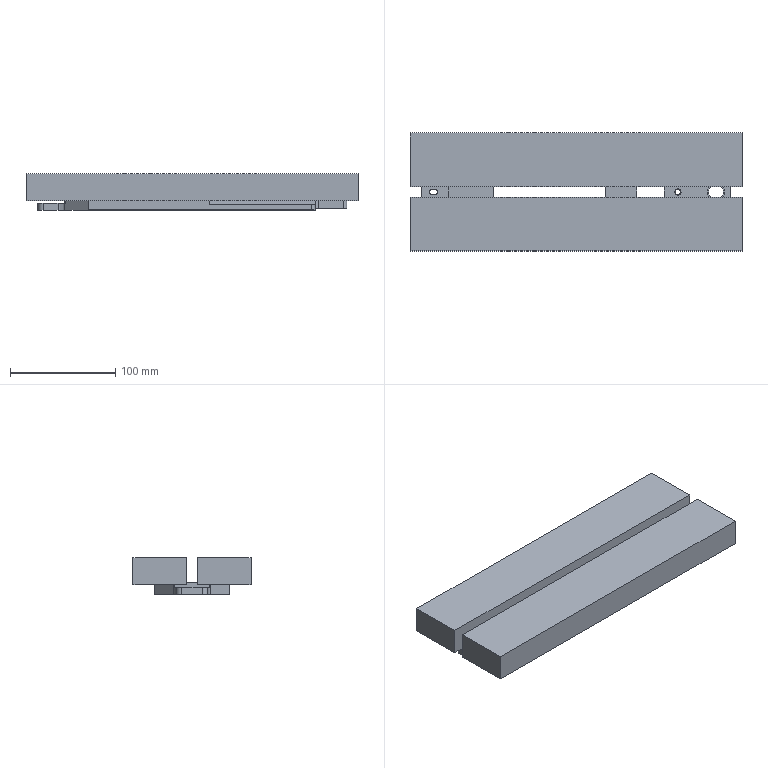NC program | NX | posted with a generic post | part box 315 x 112 x 34.85 mm
Lines 4523 to 5815 of 11462:
(PLANAR_MILL_7_COPY_1 , TOOL : D4精光)
N8984 T10 M6
N8986 G53
N8988 G17 G0 G90 X100.65 Y17.987 S4500 M3
N8990 G43 Z20. H10
N8992 Z0.3
N8994 G94 G1 Y18.214 Z0.284 F600.
N8996 X100.452 Y18.552 Z0.257
N8998 X100.114 Y18.75 Z0.229
N9000 X99.686 Z0.199
N9002 X99.349 Y18.552 Z0.172
N9004 X99.15 Y18.214 Z0.145
N9006 Y17.786 Z0.115
N9008 X99.349 Y17.448 Z0.087
N9010 X99.686 Y17.25 Z0.06
N9012 X100.114 Z0.03
N9014 X100.452 Y17.448 Z0.003
N9016 X100.65 Y17.786 Z-0.025
N9018 Y18.214 Z-0.055
N9020 X100.452 Y18.552 Z-0.082
N9022 X100.114 Y18.75 Z-0.109
N9024 X99.686 Z-0.139
N9026 X99.349 Y18.552 Z-0.167
N9028 X99.15 Y18.214 Z-0.194
N9030 Y17.786 Z-0.224
N9032 X99.349 Y17.448 Z-0.251
N9034 X99.686 Y17.25 Z-0.279
N9036 X100.114 Z-0.309
N9038 X100.452 Y17.448 Z-0.336
N9040 X100.65 Y17.786 Z-0.363
N9042 Y18.214 Z-0.393
N9044 X100.452 Y18.552 Z-0.421
N9046 X100.114 Y18.75 Z-0.448
N9048 X99.686 Z-0.478
N9050 X99.349 Y18.552 Z-0.506
N9052 X99.15 Y18.214 Z-0.533
N9054 Y17.786 Z-0.563
N9056 X99.349 Y17.448 Z-0.59
N9058 X99.686 Y17.25 Z-0.618
N9060 X100.114 Z-0.648
N9062 X100.452 Y17.448 Z-0.675
N9064 X100.65 Y17.786 Z-0.702
N9066 Y18.214 Z-0.732
N9068 X100.452 Y18.552 Z-0.76
N9070 X100.114 Y18.75 Z-0.787
N9072 X99.686 Z-0.817
N9074 X99.349 Y18.552 Z-0.844
N9076 X99.15 Y18.214 Z-0.872
N9078 Y17.786 Z-0.902
N9080 X99.349 Y17.448 Z-0.929
N9082 X99.686 Y17.25 Z-0.956
N9084 X100.114 Z-0.986
N9086 X100.452 Y17.448 Z-1.014
N9088 X100.65 Y17.786 Z-1.041
N9090 Y18.214 Z-1.071
N9092 X100.452 Y18.552 Z-1.098
N9094 X100.114 Y18.75 Z-1.126
N9096 X99.686 Z-1.156
N9098 X99.349 Y18.552 Z-1.183
N9100 X99.15 Y18.214 Z-1.21
N9102 Y17.786 Z-1.24
N9104 X99.349 Y17.448 Z-1.268
N9106 X99.686 Y17.25 Z-1.295
N9108 X100.114 Z-1.325
N9110 X100.452 Y17.448 Z-1.352
N9112 X100.65 Y17.786 Z-1.38
N9114 Y18.214 Z-1.41
N9116 X100.452 Y18.552 Z-1.437
N9118 X100.114 Y18.75 Z-1.465
N9120 X99.686 Z-1.494
N9122 X99.349 Y18.552 Z-1.522
N9124 X99.15 Y18.214 Z-1.549
N9126 Y17.786 Z-1.579
N9128 X99.349 Y17.448 Z-1.607
N9130 X99.686 Y17.25 Z-1.634
N9132 X100.114 Z-1.664
N9134 X100.452 Y17.448 Z-1.691
N9136 X100.65 Y17.786 Z-1.719
N9138 Y18.214 Z-1.749
N9140 X100.452 Y18.552 Z-1.776
N9142 X100.114 Y18.75 Z-1.803
N9144 X99.686 Z-1.833
N9146 X99.349 Y18.552 Z-1.861
N9148 X99.15 Y18.214 Z-1.888
N9150 Y17.786 Z-1.918
N9152 X99.349 Y17.448 Z-1.945
N9154 X99.686 Y17.25 Z-1.973
N9156 X100.114 Z-2.003
N9158 X100.452 Y17.448 Z-2.03
N9160 X100.65 Y17.786 Z-2.057
N9162 Y18.214 Z-2.087
N9164 X100.452 Y18.552 Z-2.115
N9166 X100.114 Y18.75 Z-2.142
N9168 X99.686 Z-2.172
N9170 X99.349 Y18.552 Z-2.199
N9172 X99.15 Y18.214 Z-2.227
N9174 Y17.786 Z-2.257
N9176 X99.349 Y17.448 Z-2.284
N9178 X99.686 Y17.25 Z-2.311
N9180 X100.114 Z-2.341
N9182 X100.452 Y17.448 Z-2.369
N9184 X100.65 Y17.786 Z-2.396
N9186 Y18.214 Z-2.426
N9188 X100.452 Y18.552 Z-2.453
N9190 X100.114 Y18.75 Z-2.481
N9192 X99.686 Z-2.511
N9194 X99.349 Y18.552 Z-2.538
N9196 X99.15 Y18.214 Z-2.566
N9198 Y17.786 Z-2.596
N9200 X99.349 Y17.448 Z-2.623
N9202 X99.686 Y17.25 Z-2.65
N9204 X100.114 Z-2.68
N9206 X100.452 Y17.448 Z-2.708
N9208 X100.65 Y17.786 Z-2.735
N9210 Y18.214 Z-2.765
N9212 X100.452 Y18.552 Z-2.792
N9214 X100.114 Y18.75 Z-2.82
N9216 X99.686 Z-2.85
N9218 X99.349 Y18.552 Z-2.877
N9220 X99.15 Y18.214 Z-2.904
N9222 Y17.786 Z-2.934
N9224 X99.349 Y17.448 Z-2.962
N9226 X99.686 Y17.25 Z-2.989
N9228 X100.114 Z-3.019
N9230 X100.452 Y17.448 Z-3.046
N9232 X100.65 Y17.786 Z-3.074
N9234 Y18.214 Z-3.104
N9236 X100.452 Y18.552 Z-3.131
N9238 X100.114 Y18.75 Z-3.158
N9240 X99.686 Z-3.188
N9242 X99.349 Y18.552 Z-3.216
N9244 X99.15 Y18.214 Z-3.243
N9246 Y17.786 Z-3.273
N9248 X99.349 Y17.448 Z-3.3
N9250 X99.686 Y17.25 Z-3.328
N9252 X100.114 Z-3.358
N9254 X100.452 Y17.448 Z-3.385
N9256 X100.65 Y17.786 Z-3.412
N9258 Y18.214 Z-3.442
N9260 X100.452 Y18.552 Z-3.47
N9262 X100.114 Y18.75 Z-3.497
N9264 X99.686 Z-3.527
N9266 X99.349 Y18.552 Z-3.555
N9268 X99.15 Y18.214 Z-3.582
N9270 Y17.786 Z-3.612
N9272 X99.349 Y17.448 Z-3.639
N9274 X99.686 Y17.25 Z-3.667
N9276 X100.114 Z-3.697
N9278 X100.452 Y17.448 Z-3.724
N9280 X100.65 Y17.786 Z-3.751
N9282 Y18.214 Z-3.781
N9284 X100.452 Y18.552 Z-3.809
N9286 X100.114 Y18.75 Z-3.836
N9288 X99.686 Z-3.866
N9290 X99.349 Y18.552 Z-3.893
N9292 X99.15 Y18.214 Z-3.921
N9294 Y17.786 Z-3.951
N9296 X99.349 Y17.448 Z-3.978
N9298 X99.686 Y17.25 Z-4.005
N9300 X100.114 Z-4.035
N9302 X100.452 Y17.448 Z-4.063
N9304 X100.65 Y17.786 Z-4.09
N9306 Y18.214 Z-4.12
N9308 X100.452 Y18.552 Z-4.147
N9310 X100.114 Y18.75 Z-4.175
N9312 X99.686 Z-4.205
N9314 X99.349 Y18.552 Z-4.232
N9316 X99.15 Y18.214 Z-4.259
N9318 Y17.786 Z-4.289
N9320 X99.349 Y17.448 Z-4.317
N9322 X99.686 Y17.25 Z-4.344
N9324 X100.114 Z-4.374
N9326 X100.452 Y17.448 Z-4.401
N9328 X100.65 Y17.786 Z-4.429
N9330 Y18.214 Z-4.459
N9332 X100.452 Y18.552 Z-4.486
N9334 X100.114 Y18.75 Z-4.514
N9336 X99.686 Z-4.543
N9338 X99.349 Y18.552 Z-4.571
N9340 X99.15 Y18.214 Z-4.598
N9342 Y17.786 Z-4.628
N9344 X99.349 Y17.448 Z-4.656
N9346 X99.686 Y17.25 Z-4.683
N9348 X100.114 Z-4.713
N9350 X100.452 Y17.448 Z-4.74
N9352 X100.65 Y17.786 Z-4.768
N9354 Y18.214 Z-4.798
N9356 X100.452 Y18.552 Z-4.825
N9358 X100.114 Y18.75 Z-4.852
N9360 X99.686 Z-4.882
N9362 X99.349 Y18.552 Z-4.91
N9364 X99.15 Y18.214 Z-4.937
N9366 Y17.786 Z-4.967
N9368 X99.349 Y17.448 Z-4.994
N9370 X99.686 Y17.25 Z-5.022
N9372 X100.114 Z-5.052
N9374 X100.452 Y17.448 Z-5.079
N9376 X100.65 Y17.786 Z-5.106
N9378 Y18.214 Z-5.136
N9380 X100.452 Y18.552 Z-5.164
N9382 X100.114 Y18.75 Z-5.191
N9384 X99.686 Z-5.221
N9386 X99.349 Y18.552 Z-5.248
N9388 X99.15 Y18.214 Z-5.276
N9390 Y17.786 Z-5.306
N9392 X99.349 Y17.448 Z-5.333
N9394 X99.686 Y17.25 Z-5.36
N9396 X100.114 Z-5.39
N9398 X100.452 Y17.448 Z-5.418
N9400 X100.65 Y17.786 Z-5.445
N9402 Y18.214 Z-5.475
N9404 X100.452 Y18.552 Z-5.502
N9406 X100.114 Y18.75 Z-5.53
N9408 X99.686 Z-5.56
N9410 X99.349 Y18.552 Z-5.587
N9412 X99.15 Y18.214 Z-5.615
N9414 Y17.786 Z-5.645
N9416 X99.349 Y17.448 Z-5.672
N9418 X99.686 Y17.25 Z-5.699
N9420 X100.114 Z-5.729
N9422 X100.452 Y17.448 Z-5.757
N9424 X100.65 Y17.786 Z-5.784
N9426 Y18.214 Z-5.814
N9428 X100.452 Y18.552 Z-5.841
N9430 X100.114 Y18.75 Z-5.869
N9432 X99.686 Z-5.899
N9434 X99.349 Y18.552 Z-5.926
N9436 X99.15 Y18.214 Z-5.953
N9438 Y17.786 Z-5.983
N9440 X99.349 Y17.448 Z-6.011
N9442 X99.686 Y17.25 Z-6.038
N9444 X100.114 Z-6.068
N9446 X100.452 Y17.448 Z-6.095
N9448 X100.65 Y17.786 Z-6.123
N9450 Y18.214 Z-6.153
N9452 X100.452 Y18.552 Z-6.18
N9454 X100.114 Y18.75 Z-6.207
N9456 X99.686 Z-6.237
N9458 X99.349 Y18.552 Z-6.265
N9460 X99.15 Y18.214 Z-6.292
N9462 Y17.786 Z-6.322
N9464 X99.349 Y17.448 Z-6.349
N9466 X99.686 Y17.25 Z-6.377
N9468 X100.114 Z-6.407
N9470 X100.452 Y17.448 Z-6.434
N9472 X100.65 Y17.786 Z-6.462
N9474 Y18.214 Z-6.491
N9476 X100.452 Y18.552 Z-6.519
N9478 X100.114 Y18.75 Z-6.546
N9480 X99.686 Z-6.576
N9482 X99.349 Y18.552 Z-6.604
N9484 X99.15 Y18.214 Z-6.631
N9486 Y17.786 Z-6.661
N9488 X99.349 Y17.448 Z-6.688
N9490 X99.686 Y17.25 Z-6.716
N9492 X100.114 Z-6.746
N9494 X100.452 Y17.448 Z-6.773
N9496 X100.65 Y17.786 Z-6.8
N9498 Y18.214 Z-6.83
N9500 X100.452 Y18.552 Z-6.858
N9502 X100.114 Y18.75 Z-6.885
N9504 X99.686 Z-6.915
N9506 X99.349 Y18.552 Z-6.942
N9508 X99.15 Y18.214 Z-6.97
N9510 Y17.786 Z-7.
N9512 X99.349 Y17.448 Z-7.027
N9514 X99.686 Y17.25 Z-7.054
N9516 X100.114 Z-7.084
N9518 X100.452 Y17.448 Z-7.112
N9520 X100.65 Y17.786 Z-7.139
N9522 Y18.214 Z-7.169
N9524 X100.452 Y18.552 Z-7.196
N9526 X100.114 Y18.75 Z-7.224
N9528 X99.686 Z-7.254
N9530 X99.349 Y18.552 Z-7.281
N9532 X99.15 Y18.214 Z-7.308
N9534 Y17.786 Z-7.338
N9536 X99.349 Y17.448 Z-7.366
N9538 X99.686 Y17.25 Z-7.393
N9540 X100.114 Z-7.423
N9542 X100.452 Y17.448 Z-7.45
N9544 X100.65 Y17.786 Z-7.478
N9546 Y18.214 Z-7.508
N9548 X100.452 Y18.552 Z-7.535
N9550 X100.114 Y18.75 Z-7.563
N9552 X99.686 Z-7.593
N9554 X99.349 Y18.552 Z-7.62
N9556 X99.15 Y18.214 Z-7.647
N9558 Y17.786 Z-7.677
N9560 X99.349 Y17.448 Z-7.705
N9562 X99.686 Y17.25 Z-7.732
N9564 X100.114 Z-7.762
N9566 X100.452 Y17.448 Z-7.789
N9568 X100.65 Y17.786 Z-7.817
N9570 Y18.214 Z-7.847
N9572 X100.452 Y18.552 Z-7.874
N9574 X100.114 Y18.75 Z-7.901
N9576 X99.686 Z-7.931
N9578 X99.349 Y18.552 Z-7.959
N9580 X99.15 Y18.214 Z-7.986
N9582 Y17.786 Z-8.016
N9584 X99.349 Y17.448 Z-8.043
N9586 X99.686 Y17.25 Z-8.071
N9588 X100.114 Z-8.101
N9590 X100.452 Y17.448 Z-8.128
N9592 X100.65 Y17.786 Z-8.155
N9594 Y18.214 Z-8.185
N9596 X100.452 Y18.552 Z-8.213
N9598 X100.114 Y18.75 Z-8.24
N9600 X99.686 Z-8.27
N9602 X99.349 Y18.552 Z-8.297
N9604 X99.15 Y18.214 Z-8.325
N9606 Y17.786 Z-8.355
N9608 X99.349 Y17.448 Z-8.382
N9610 X99.686 Y17.25 Z-8.409
N9612 X100.114 Z-8.439
N9614 X100.452 Y17.448 Z-8.467
N9616 X100.65 Y17.786 Z-8.494
N9618 Y18.214 Z-8.524
N9620 X100.452 Y18.552 Z-8.552
N9622 X100.114 Y18.75 Z-8.579
N9624 X99.686 Z-8.609
N9626 X99.349 Y18.552 Z-8.636
N9628 X99.15 Y18.214 Z-8.664
N9630 Y17.786 Z-8.694
N9632 X99.349 Y17.448 Z-8.721
N9634 X99.686 Y17.25 Z-8.748
N9636 X100.114 Z-8.778
N9638 X100.452 Y17.448 Z-8.806
N9640 X100.65 Y17.786 Z-8.833
N9642 Y18.214 Z-8.863
N9644 X100.452 Y18.552 Z-8.89
N9646 X100.114 Y18.75 Z-8.918
N9648 X99.686 Z-8.948
N9650 X99.349 Y18.552 Z-8.975
N9652 X99.15 Y18.214 Z-9.002
N9654 Y17.786 Z-9.032
N9656 X99.349 Y17.448 Z-9.06
N9658 X99.686 Y17.25 Z-9.087
N9660 X100.114 Z-9.117
N9662 X100.452 Y17.448 Z-9.144
N9664 X100.65 Y17.786 Z-9.172
N9666 Y18.214 Z-9.202
N9668 X100.452 Y18.552 Z-9.229
N9670 X100.114 Y18.75 Z-9.256
N9672 X99.686 Z-9.286
N9674 X99.349 Y18.552 Z-9.314
N9676 X99.15 Y18.214 Z-9.341
N9678 Y17.786 Z-9.371
N9680 X99.349 Y17.448 Z-9.398
N9682 X99.686 Y17.25 Z-9.426
N9684 X100.114 Z-9.456
N9686 X100.452 Y17.448 Z-9.483
N9688 X100.65 Y17.786 Z-9.511
N9690 Y18.214 Z-9.54
N9692 X100.452 Y18.552 Z-9.568
N9694 X100.114 Y18.75 Z-9.595
N9696 X99.686 Z-9.625
N9698 X99.349 Y18.552 Z-9.653
N9700 X99.15 Y18.214 Z-9.68
N9702 Y17.786 Z-9.71
N9704 X99.349 Y17.448 Z-9.737
N9706 X99.686 Y17.25 Z-9.765
N9708 X100.114 Z-9.795
N9710 X100.452 Y17.448 Z-9.822
N9712 X100.65 Y17.786 Z-9.849
N9714 Y18.214 Z-9.879
N9716 X100.452 Y18.552 Z-9.907
N9718 X100.114 Y18.75 Z-9.934
N9720 X99.686 Z-9.964
N9722 X99.349 Y18.552 Z-9.991
N9724 X99.15 Y18.214 Z-10.019
N9726 Y17.786 Z-10.049
N9728 X99.349 Y17.448 Z-10.076
N9730 X99.686 Y17.25 Z-10.103
N9732 X100.114 Z-10.133
N9734 X100.452 Y17.448 Z-10.161
N9736 X100.65 Y17.786 Z-10.188
N9738 Y18.214 Z-10.218
N9740 X100.452 Y18.552 Z-10.245
N9742 X100.114 Y18.75 Z-10.273
N9744 X99.686 Z-10.303
N9746 X99.349 Y18.552 Z-10.33
N9748 X99.15 Y18.214 Z-10.357
N9750 Y17.786 Z-10.387
N9752 X99.349 Y17.448 Z-10.415
N9754 X99.686 Y17.25 Z-10.442
N9756 X100.114 Z-10.472
N9758 X100.452 Y17.448 Z-10.499
N9760 X100.65 Y17.786 Z-10.527
N9762 Y18.214 Z-10.557
N9764 X100.452 Y18.552 Z-10.584
N9766 X100.114 Y18.75 Z-10.612
N9768 X99.686 Z-10.642
N9770 X99.349 Y18.552 Z-10.669
N9772 X99.15 Y18.214 Z-10.696
N9774 Y17.786 Z-10.726
N9776 X99.349 Y17.448 Z-10.754
N9778 X99.686 Y17.25 Z-10.781
N9780 X100.114 Z-10.811
N9782 X100.452 Y17.448 Z-10.838
N9784 X100.65 Y17.786 Z-10.866
N9786 Y18.214 Z-10.896
N9788 X100.452 Y18.552 Z-10.923
N9790 X100.114 Y18.75 Z-10.95
N9792 X99.686 Z-10.98
N9794 X99.349 Y18.552 Z-11.008
N9796 X99.15 Y18.214 Z-11.035
N9798 Y18. Z-11.05
N9800 G3 X99.9 Y17.25 R0.75
N9802 X99.15 Y18. R-0.75
N9804 G1 Z-10.75
N9806 G0 Z20.
N9808 M5
(PLANAR_MILL_1 , TOOL : D6精光)
N9810 T09 M6
N9812 G53
N9814 G17 G0 G90 X115.623 Y-41.542 S5500 M3
N9816 G43 Z20. H9
N9818 Z-8.85
N9820 G94 G1 Z-11.85 F1000.
N9822 G41 X115.71 Y-41.05 D9
N9824 G3 X113.71 Y-39.05 R2.
N9826 G1 X-98.29
N9828 G2 X-100.252 Y-38.335 R3.05
N9830 G1 X-122.641 Y-19.528
N9832 G3 X-127.111 Y-17.9 R6.95
N9834 G1 X-141.29
N9836 G2 X-149.34 Y-9.85 R8.05
N9838 G1 Y9.85
N9840 G2 X-141.29 Y17.9 R8.05
N9842 G1 X-127.111
N9844 G3 X-122.641 Y19.528 R6.95
N9846 G1 X-100.252 Y38.335
N9848 G2 X-98.29 Y39.05 R3.05
N9850 G1 X113.71
N9852 G2 X119.76 Y33. R6.05
N9854 G1 Y15.55
N9856 X143.71
N9858 G2 X149.76 Y9.5 R6.05
N9860 G1 Y-9.5
N9862 G2 X143.71 Y-15.55 R6.05
N9864 G1 X119.76
N9866 Y-33.
N9868 G2 X113.71 Y-39.05 R6.05
N9870 G3 X111.71 Y-41.05 R2.
N9872 G40
N9874 G1 X111.797 Y-41.542
N9876 X115.623 Y-41.492
N9878 G41 X115.71 Y-41.
N9880 G3 X113.71 Y-39. R2.
N9882 G1 X-98.29
N9884 G2 X-100.22 Y-38.297 R3.
N9886 G1 X-122.609 Y-19.49
N9888 G3 X-127.111 Y-17.85 R7.
N9890 G1 X-141.29
N9892 G2 X-149.29 Y-9.85 R8.
N9894 G1 Y9.85
N9896 G2 X-141.29 Y17.85 R8.
N9898 G1 X-127.111
N9900 G3 X-122.609 Y19.49 R7.
N9902 G1 X-100.22 Y38.297
N9904 G2 X-98.29 Y39. R3.
N9906 G1 X113.71
N9908 G2 X119.71 Y33. R6.
N9910 G1 Y15.5
N9912 X143.71
N9914 G2 X149.71 Y9.5 R6.
N9916 G1 Y-9.5
N9918 G2 X143.71 Y-15.5 R6.
N9920 G1 X119.71
N9922 Y-33.
N9924 G2 X113.71 Y-39. R6.
N9926 G3 X111.71 Y-41. R2.
N9928 G1 Y-41.05
N9930 G40
N9932 X111.797 Y-41.542
N9934 Z-8.85
N9936 G0 Z20.
(PLANAR_MILL_1_COPY , TOOL : D6精光)
N9938 X130.374 Y0.913 H29
N9940 Z-8.85
N9942 G1 Z-11.85 F100.
N9944 G41 X129.882 Y1. D29
N9946 X129.71
N9948 G3 X128.71 Y0. R1.
N9950 X132.71 Y-4. R4.
N9952 X128.71 Y0. R-4.
N9954 X129.71 Y-1. R1.
N9956 G40
N9958 G1 X130.202 Y-0.913
N9960 Y0.913
N9962 G41 X129.71 Y1.
N9964 G3 X128.71 Y0. R1.
N9966 X132.71 Y-4. R4.
N9968 X128.71 Y0. R-4.
N9970 X129.71 Y-1. R1.
N9972 G1 X129.882
N9974 G40
N9976 X130.374 Y-0.913
N9978 Z-8.85
N9980 G0 Z20.
(PLANAR_MILL_1_COPY_COPY_1 , TOOL : D6精光)
N9982 X18.643 Y20.424 H9
N9984 Z-8.85
N9986 G1 Z-11.85 F600.
N9988 G41 X18.73 Y20.916 D9
N9990 Y21.
N9992 G3 X17.73 Y22. R1.
N9994 G1 X-68.31
N9996 G3 X-75.31 Y15. R7.
N9998 G1 Y-15.
N10000 G3 X-68.31 Y-22. R7.
N10002 G1 X17.73
N10004 G3 X24.73 Y-15. R7.
N10006 G1 Y15.
N10008 G3 X17.73 Y22. R7.
N10010 X16.73 Y21. R1.
N10012 G40
N10014 G1 X16.817 Y20.508
N10016 Z-8.85
N10018 G0 Z20.
(PLANAR_MILL_1_COPY_COPY , TOOL : D6精光)
N10020 X129.092 Y0.913
N10022 Z-1.
N10024 G1 Z-4. F100.
N10026 G41 X128.6 Y1.
N10028 X128.48
N10030 G3 X127.48 Y0. R1.
N10032 X132.71 Y-5.23 R5.23
N10034 X127.48 Y0. R-5.23
N10036 X128.48 Y-1. R1.
N10038 G40
N10040 G1 X128.972 Y-0.913
N10042 X128.952 Y0.913
N10044 G41 X128.46 Y1.
N10046 G3 X127.46 Y0. R1.
N10048 X132.71 Y-5.25 R5.25
N10050 X127.46 Y0. R-5.25
N10052 X128.46 Y-1. R1.
N10054 G1 X128.579
N10056 G40
N10058 X129.072 Y-0.913
N10060 Z-1.
N10062 G0 Z20.
(FLOOR_WALL , TOOL : D6精光)
N10064 X101.257 Y41.
N10066 Z-2.
N10068 G1 Z-5. F600.
N10070 Y34.5
N10072 X113.71
N10074 G2 X115.21 Y33. R1.5
N10076 G1 Y21.171
N10078 X41.898 Y34.5
N10080 X101.257
N10082 Y30.
N10084 X110.71
N10086 Y26.563
N10088 X91.804 Y30.
N10090 X89.206 Y31.5
N10092 X75.169
N10094 X88.979 Y28.989
N10096 G2 X89.206 Y31.5 R3.
N10098 G1 X91.804 Y30.
N10100 X101.257
N10102 X102.257
N10104 Y41.
N10106 Z-2.
N10108 G0 Z20.
N10110 X101.257 Y-41.
N10112 Z-2.
N10114 G1 Z-5.
N10116 Y-34.5
N10118 X41.898
N10120 X115.21 Y-21.171
N10122 Y-33.
N10124 G2 X113.71 Y-34.5 R1.5
N10126 G1 X101.257
N10128 Y-30.
N10130 X91.804
N10132 X88.979 Y-28.989
N10134 X75.169 Y-31.5
N10136 X89.206
N10138 G2 X88.979 Y-28.989 R3.
N10140 G1 X91.804 Y-30.
N10142 X110.71 Y-26.563
N10144 Y-30.
N10146 X101.257
N10148 X100.257
N10150 Y-41.
N10152 Z-2.
N10154 G0 Z20.
(PLANAR_MILL_6 , TOOL : D6精光)
N10156 X12.842 Y39.841
N10158 Z-1.995
N10160 G1 Z-4.995 F800.
N10162 G41 X13.311 Y39.667
N10164 X17.247 Y38.952
N10166 X117.247 Y20.77
N10168 X121.182 Y20.054
N10170 G40
N10172 X121.682 Y20.052
N10174 Z-1.995
N10176 G0 Z20.
N10178 Y-20.052
N10180 Z-1.995
N10182 G1 Z-4.995
N10184 G41 X121.182 Y-20.054
N10186 X117.247 Y-20.77
N10188 X17.247 Y-38.952
N10190 X13.311 Y-39.667
N10192 G40
N10194 X12.842 Y-39.841
N10196 Z-1.995
N10198 G0 Z20.
(FLOOR_WALL_1 , TOOL : D6精光)
N10200 X-151.29 Y0.
N10202 Z-1.
N10204 G1 Z-4. F600.
N10206 X-144.79
N10208 Y9.85
N10210 G2 X-141.29 Y13.35 R3.5
N10212 G1 X-127.111
N10214 G3 X-123.5 Y13.932 R11.5
N10216 G1 Y-13.932
N10218 G3 X-127.111 Y-13.35 R11.5
N10220 G1 X-141.29
N10222 G2 X-144.79 Y-9.85 R3.5
N10224 G1 Y0.
N10226 X-140.29
N10228 Y8.85
N10230 X-128.
N10232 Y-8.85
N10234 X-140.29
N10236 Y0.
N10238 X-135.79
N10240 Y4.35
N10242 X-132.5
N10244 Y-4.35
N10246 X-135.79
N10248 Y0.
N10250 Y1.
N10252 X-137.79
N10254 Z-1.
N10256 G0 Z20.
(PLANAR_MILL_6_COPY , TOOL : D6精光)
N10258 X-121.854 Y-23.379
N10260 Z-0.995
N10262 G1 Z-3.995 F800.
N10264 G41 X-121.471 Y-23.058
N10266 G3 X-121.716 Y-20.24 R2.
N10268 G2 X-123.5 Y-16.412 R5.
N10270 G1 Y16.412
N10272 G2 X-121.716 Y20.24 R5.
N10274 G3 X-121.471 Y23.058 R2.
N10276 G40
N10278 G1 X-121.854 Y23.379
N10280 Z-0.995
N10282 G0 Z20.
(PLANAR_MILL_1_COPY_1 , TOOL : D6精光)
N10284 X-139.377 Y-20.392
N10286 Z-8.85
N10288 G1 Z-11.85 F1000.
N10290 G41 X-139.29 Y-19.9
N10292 G3 X-141.29 Y-17.9 R2.
N10294 G2 X-149.34 Y-9.85 R8.05
N10296 G1 Y9.85
N10298 G2 X-141.29 Y17.9 R8.05
N10300 G3 X-139.29 Y19.9 R2.
N10302 G40
N10304 G1 X-139.377 Y20.392
N10306 Z-8.85
N10308 G0 Z20.
N10310 Y-20.392
N10312 Z-8.85
N10314 G1 Z-11.85
N10316 G41 X-139.29 Y-19.9
N10318 Y-19.85
N10320 G3 X-141.29 Y-17.85 R2.
N10322 G2 X-149.29 Y-9.85 R8.
N10324 G1 Y9.85
N10326 G2 X-141.29 Y17.85 R8.
N10328 G3 X-139.29 Y19.85 R2.
N10330 G1 Y19.9
N10332 G40
N10334 X-139.377 Y20.392
N10336 Z-8.85
N10338 G0 Z20.
N10340 M5
(PLANAR_MILL_7 , TOOL : D4精光)
N10342 T10 M6
N10344 G53
N10346 G17 G0 G90 X96.27 Y-0.151 S4500 M3
N10348 G43 Z20. H10
N10350 Z-0.2
N10352 G94 G1 Y-0.165 Z-0.201 F600.
N10354 X96.545 Y-0.44 Z-0.228
N10356 X96.875 Z-0.251
N10358 X97.15 Y-0.165 Z-0.278
N10360 Y0.165 Z-0.302
N10362 X96.875 Y0.44 Z-0.329
N10364 X96.545 Z-0.352
N10366 X96.27 Y0.165 Z-0.379
N10368 Y-0.165 Z-0.402
N10370 X96.545 Y-0.44 Z-0.429
N10372 X96.875 Z-0.452
N10374 X97.15 Y-0.165 Z-0.48
N10376 Y0.165 Z-0.503
N10378 X96.875 Y0.44 Z-0.53
N10380 X96.545 Z-0.553
N10382 X96.27 Y0.165 Z-0.58
N10384 Y-0.165 Z-0.603
N10386 X96.545 Y-0.44 Z-0.63
N10388 X96.875 Z-0.654
N10390 X97.15 Y-0.165 Z-0.681
N10392 Y0.165 Z-0.704
N10394 X96.875 Y0.44 Z-0.731
N10396 X96.545 Z-0.754
N10398 X96.27 Y0.165 Z-0.781
N10400 Y-0.165 Z-0.804
N10402 X96.545 Y-0.44 Z-0.832
N10404 X96.875 Z-0.855
N10406 X97.15 Y-0.165 Z-0.882
N10408 Y0.165 Z-0.905
N10410 X96.875 Y0.44 Z-0.932
N10412 X96.545 Z-0.955
N10414 X96.27 Y0.165 Z-0.982
N10416 Y-0.165 Z-1.005
N10418 X96.545 Y-0.44 Z-1.033
N10420 X96.875 Z-1.056
N10422 X97.15 Y-0.165 Z-1.083
N10424 Y0.165 Z-1.106
N10426 X96.875 Y0.44 Z-1.133
N10428 X96.545 Z-1.156
N10430 X96.27 Y0.165 Z-1.184
N10432 Y-0.165 Z-1.207
N10434 X96.545 Y-0.44 Z-1.234
N10436 X96.875 Z-1.257
N10438 X97.15 Y-0.165 Z-1.284
N10440 Y0.165 Z-1.307
N10442 X96.875 Y0.44 Z-1.334
N10444 X96.545 Z-1.357
N10446 X96.27 Y0.165 Z-1.385
N10448 Y-0.165 Z-1.408
N10450 X96.545 Y-0.44 Z-1.435
N10452 X96.875 Z-1.458
N10454 X97.15 Y-0.165 Z-1.485
N10456 Y0.165 Z-1.508
N10458 X96.875 Y0.44 Z-1.535
N10460 X96.545 Z-1.559
N10462 X96.27 Y0.165 Z-1.586
N10464 Y-0.165 Z-1.609
N10466 X96.545 Y-0.44 Z-1.636
N10468 X96.875 Z-1.659
N10470 X97.15 Y-0.165 Z-1.686
N10472 Y0.165 Z-1.709
N10474 X96.875 Y0.44 Z-1.737
N10476 X96.545 Z-1.76
N10478 X96.27 Y0.165 Z-1.787
N10480 Y-0.165 Z-1.81
N10482 X96.545 Y-0.44 Z-1.837
N10484 X96.875 Z-1.86
N10486 X97.15 Y-0.165 Z-1.887
N10488 Y0.165 Z-1.911
N10490 X96.875 Y0.44 Z-1.938
N10492 X96.545 Z-1.961
N10494 X96.27 Y0.165 Z-1.988
N10496 Y-0.165 Z-2.011
N10498 X96.545 Y-0.44 Z-2.038
N10500 X96.875 Z-2.061
N10502 X97.15 Y-0.165 Z-2.089
N10504 Y0.165 Z-2.112
N10506 X96.875 Y0.44 Z-2.139
N10508 X96.545 Z-2.162
N10510 X96.27 Y0.165 Z-2.189
N10512 Y-0.165 Z-2.212
N10514 X96.545 Y-0.44 Z-2.239
N10516 X96.875 Z-2.263
N10518 X97.15 Y-0.165 Z-2.29
N10520 Y0.165 Z-2.313
N10522 X96.875 Y0.44 Z-2.34
N10524 X96.545 Z-2.363
N10526 X96.27 Y0.165 Z-2.39
N10528 Y-0.165 Z-2.413
N10530 X96.545 Y-0.44 Z-2.441
N10532 X96.875 Z-2.464
N10534 X97.15 Y-0.165 Z-2.491
N10536 Y0.165 Z-2.514
N10538 X96.875 Y0.44 Z-2.541
N10540 X96.545 Z-2.564
N10542 X96.27 Y0.165 Z-2.591
N10544 Y-0.165 Z-2.614
N10546 X96.545 Y-0.44 Z-2.642
N10548 X96.875 Z-2.665
N10550 X97.15 Y-0.165 Z-2.692
N10552 Y0.165 Z-2.715
N10554 X96.875 Y0.44 Z-2.742
N10556 X96.545 Z-2.765
N10558 X96.27 Y0.165 Z-2.792
N10560 Y-0.165 Z-2.816
N10562 X96.545 Y-0.44 Z-2.843
N10564 X96.875 Z-2.866
N10566 X97.15 Y-0.165 Z-2.893
N10568 Y0.165 Z-2.916
N10570 X96.875 Y0.44 Z-2.943
N10572 X96.545 Z-2.966
N10574 X96.27 Y0.165 Z-2.994
N10576 Y-0.165 Z-3.017
N10578 X96.545 Y-0.44 Z-3.044
N10580 X96.875 Z-3.067
N10582 X97.15 Y-0.165 Z-3.094
N10584 Y0.165 Z-3.117
N10586 X96.875 Y0.44 Z-3.144
N10588 X96.545 Z-3.168
N10590 X96.27 Y0.165 Z-3.195
N10592 Y-0.165 Z-3.218
N10594 X96.545 Y-0.44 Z-3.245
N10596 X96.875 Z-3.268
N10598 X97.15 Y-0.165 Z-3.295
N10600 Y0.165 Z-3.318
N10602 X96.875 Y0.44 Z-3.346
N10604 X96.545 Z-3.369
N10606 X96.27 Y0.165 Z-3.396
N10608 Y-0.165 Z-3.419
N10610 X96.545 Y-0.44 Z-3.446
N10612 X96.875 Z-3.469
N10614 X97.15 Y-0.165 Z-3.496
N10616 Y0.165 Z-3.52
N10618 X96.875 Y0.44 Z-3.547
N10620 X96.545 Z-3.57
N10622 X96.27 Y0.165 Z-3.597
N10624 Y-0.165 Z-3.62
N10626 X96.545 Y-0.44 Z-3.647
N10628 X96.875 Z-3.67
N10630 X97.15 Y-0.165 Z-3.698
N10632 Y0.165 Z-3.721
N10634 X96.875 Y0.44 Z-3.748
N10636 X96.545 Z-3.771
N10638 X96.27 Y0.165 Z-3.798
N10640 Y-0.165 Z-3.821
N10642 X96.545 Y-0.44 Z-3.848
N10644 X96.875 Z-3.871
N10646 X97.15 Y-0.165 Z-3.899
N10648 Y0.165 Z-3.922
N10650 X96.875 Y0.44 Z-3.949
N10652 X96.545 Z-3.972
N10654 X96.27 Y0.165 Z-3.999
N10656 Y-0.165 Z-4.022
N10658 X96.545 Y-0.44 Z-4.049
N10660 X96.875 Z-4.073
N10662 X97.15 Y-0.165 Z-4.1
N10664 Y0.165 Z-4.123
N10666 X96.875 Y0.44 Z-4.15
N10668 X96.545 Z-4.173
N10670 X96.27 Y0.165 Z-4.2
N10672 Y-0.165 Z-4.223
N10674 X96.545 Y-0.44 Z-4.251
N10676 X96.875 Z-4.274
N10678 X97.15 Y-0.165 Z-4.301
N10680 Y0.165 Z-4.324
N10682 X96.875 Y0.44 Z-4.351
N10684 X96.545 Z-4.374
N10686 X96.27 Y0.165 Z-4.401
N10688 Y-0.165 Z-4.425
N10690 X96.545 Y-0.44 Z-4.452
N10692 X96.875 Z-4.475
N10694 X97.15 Y-0.165 Z-4.502
N10696 Y0.165 Z-4.525
N10698 X96.875 Y0.44 Z-4.552
N10700 X96.545 Z-4.575
N10702 X96.27 Y0.165 Z-4.603
N10704 Y-0.165 Z-4.626
N10706 X96.545 Y-0.44 Z-4.653
N10708 X96.875 Z-4.676
N10710 X97.15 Y-0.165 Z-4.703
N10712 Y0.165 Z-4.726
N10714 X96.875 Y0.44 Z-4.753
N10716 X96.545 Z-4.777
N10718 X96.27 Y0.165 Z-4.804
N10720 Y-0.165 Z-4.827
N10722 X96.545 Y-0.44 Z-4.854
N10724 X96.875 Z-4.877
N10726 X97.15 Y-0.165 Z-4.904
N10728 Y0.165 Z-4.927
N10730 X96.875 Y0.44 Z-4.955
N10732 X96.545 Z-4.978
N10734 X96.27 Y0.165 Z-5.005
N10736 Y-0.165 Z-5.028
N10738 X96.545 Y-0.44 Z-5.055
N10740 X96.875 Z-5.078
N10742 X97.15 Y-0.165 Z-5.105
N10744 Y0.165 Z-5.128
N10746 X96.875 Y0.44 Z-5.156
N10748 X96.545 Z-5.179
N10750 X96.27 Y0.165 Z-5.206
N10752 Y-0.165 Z-5.229
N10754 X96.545 Y-0.44 Z-5.256
N10756 X96.875 Z-5.279
N10758 X97.15 Y-0.165 Z-5.306
N10760 Y0.165 Z-5.33
N10762 X96.875 Y0.44 Z-5.357
N10764 X96.545 Z-5.38
N10766 X96.27 Y0.165 Z-5.407
N10768 Y-0.165 Z-5.43
N10770 X96.545 Y-0.44 Z-5.457
N10772 X96.875 Z-5.48
N10774 X97.15 Y-0.165 Z-5.508
N10776 Y0.165 Z-5.531
N10778 X96.875 Y0.44 Z-5.558
N10780 X96.545 Z-5.581
N10782 X96.27 Y0.165 Z-5.608
N10784 Y-0.165 Z-5.631
N10786 X96.545 Y-0.44 Z-5.658
N10788 X96.875 Z-5.682
N10790 X97.15 Y-0.165 Z-5.709
N10792 Y0.165 Z-5.732
N10794 X96.875 Y0.44 Z-5.759
N10796 X96.545 Z-5.782
N10798 X96.27 Y0.165 Z-5.809
N10800 Y-0.165 Z-5.832
N10802 X96.545 Y-0.44 Z-5.86
N10804 X96.875 Z-5.883
N10806 X97.15 Y-0.165 Z-5.91
N10808 Y0.165 Z-5.933
N10810 X96.875 Y0.44 Z-5.96
N10812 X96.545 Z-5.983
N10814 X96.27 Y0.165 Z-6.01
N10816 Y-0.165 Z-6.034
N10818 X96.545 Y-0.44 Z-6.061
N10820 X96.875 Z-6.084
N10822 X97.15 Y-0.165 Z-6.111
N10824 Y0.165 Z-6.134
N10826 X96.875 Y0.44 Z-6.161
N10828 X96.545 Z-6.184
N10830 X96.27 Y0.165 Z-6.212
N10832 Y-0.165 Z-6.235
N10834 X96.545 Y-0.44 Z-6.262
N10836 X96.875 Z-6.285
N10838 X97.15 Y-0.165 Z-6.312
N10840 Y0.165 Z-6.335
N10842 X96.875 Y0.44 Z-6.362
N10844 X96.545 Z-6.385
N10846 X96.27 Y0.165 Z-6.413
N10848 Y-0.165 Z-6.436
N10850 X96.545 Y-0.44 Z-6.463
N10852 X96.875 Z-6.486
N10854 X97.15 Y-0.165 Z-6.513
N10856 Y0.165 Z-6.536
N10858 X96.875 Y0.44 Z-6.564
N10860 X96.545 Z-6.587
N10862 X96.27 Y0.165 Z-6.614
N10864 Y-0.165 Z-6.637
N10866 X96.545 Y-0.44 Z-6.664
N10868 X96.875 Z-6.687
N10870 X97.15 Y-0.165 Z-6.714
N10872 Y0.165 Z-6.737
N10874 X96.875 Y0.44 Z-6.765
N10876 X96.545 Z-6.788
N10878 X96.27 Y0.165 Z-6.815
N10880 Y-0.165 Z-6.838
N10882 X96.545 Y-0.44 Z-6.865
N10884 X96.875 Z-6.888
N10886 X97.15 Y-0.165 Z-6.915
N10888 Y0.165 Z-6.939
N10890 X96.875 Y0.44 Z-6.966
N10892 X96.545 Z-6.989
N10894 X96.27 Y0.165 Z-7.016
N10896 Y-0.165 Z-7.039
N10898 X96.545 Y-0.44 Z-7.066
N10900 X96.875 Z-7.089
N10902 X97.15 Y-0.165 Z-7.117
N10904 Y0.165 Z-7.14
N10906 X96.875 Y0.44 Z-7.167
N10908 X96.545 Z-7.19
N10910 X96.27 Y0.165 Z-7.217
N10912 Y-0.165 Z-7.24
N10914 X96.545 Y-0.44 Z-7.267
N10916 X96.875 Z-7.291
N10918 X97.15 Y-0.165 Z-7.318
N10920 Y0.165 Z-7.341
N10922 X96.875 Y0.44 Z-7.368
N10924 X96.545 Z-7.391
N10926 X96.27 Y0.165 Z-7.418
N10928 Y-0.165 Z-7.441
N10930 X96.545 Y-0.44 Z-7.469
N10932 X96.875 Z-7.492
N10934 X97.15 Y-0.165 Z-7.519
N10936 Y0.165 Z-7.542
N10938 X96.875 Y0.44 Z-7.569
N10940 X96.545 Z-7.592
N10942 X96.27 Y0.165 Z-7.619
N10944 Y-0.165 Z-7.642
N10946 X96.545 Y-0.44 Z-7.67
N10948 X96.875 Z-7.693
N10950 X97.15 Y-0.165 Z-7.72
N10952 Y0.165 Z-7.743
N10954 X96.875 Y0.44 Z-7.77
N10956 X96.545 Z-7.793
N10958 X96.27 Y0.165 Z-7.821
N10960 Y-0.165 Z-7.844
N10962 X96.545 Y-0.44 Z-7.871
N10964 X96.875 Z-7.894
N10966 X97.15 Y-0.165 Z-7.921
N10968 Y0.165 Z-7.944
N10970 X96.875 Y0.44 Z-7.971
N10972 X96.545 Z-7.994
N10974 X96.27 Y0.165 Z-8.022
N10976 Y-0.165 Z-8.045
N10978 X96.545 Y-0.44 Z-8.072
N10980 X96.875 Z-8.095
N10982 X97.15 Y-0.165 Z-8.122
N10984 Y0.165 Z-8.145
N10986 X96.875 Y0.44 Z-8.172
N10988 X96.545 Z-8.196
N10990 X96.27 Y0.165 Z-8.223
N10992 Y-0.165 Z-8.246
N10994 X96.545 Y-0.44 Z-8.273
N10996 X96.875 Z-8.296
N10998 X97.15 Y-0.165 Z-8.323
N11000 Y0.165 Z-8.346
N11002 X96.875 Y0.44 Z-8.374
N11004 X96.545 Z-8.397
N11006 X96.27 Y0.165 Z-8.424
N11008 Y-0.165 Z-8.447
N11010 X96.545 Y-0.44 Z-8.474
N11012 X96.875 Z-8.497
N11014 X97.15 Y-0.165 Z-8.524
N11016 Y0.165 Z-8.548
N11018 X96.875 Y0.44 Z-8.575
N11020 X96.545 Z-8.598
N11022 X96.27 Y0.165 Z-8.625
N11024 Y-0.165 Z-8.648
N11026 X96.545 Y-0.44 Z-8.675
N11028 X96.875 Z-8.698
N11030 X97.15 Y-0.165 Z-8.726
N11032 Y0.165 Z-8.749
N11034 X96.875 Y0.44 Z-8.776
N11036 X96.545 Z-8.799
N11038 X96.27 Y0.165 Z-8.826
N11040 Y-0.165 Z-8.849
N11042 X96.545 Y-0.44 Z-8.876
N11044 X96.875 Z-8.9
N11046 X97.15 Y-0.165 Z-8.927
N11048 Y0.165 Z-8.95
N11050 X96.875 Y0.44 Z-8.977
N11052 X96.545 Z-9.
N11054 X96.27 Y0.165 Z-9.027
N11056 Y-0.165 Z-9.05
N11058 X96.545 Y-0.44 Z-9.078
N11060 X96.875 Z-9.101
N11062 X97.15 Y-0.165 Z-9.128
N11064 Y0.165 Z-9.151
N11066 X96.875 Y0.44 Z-9.178
N11068 X96.545 Z-9.201
N11070 X96.27 Y0.165 Z-9.228
N11072 Y-0.165 Z-9.251
N11074 X96.545 Y-0.44 Z-9.279
N11076 X96.875 Z-9.302
N11078 X97.15 Y-0.165 Z-9.329
N11080 Y0.165 Z-9.352
N11082 X96.875 Y0.44 Z-9.379
N11084 X96.545 Z-9.402
N11086 X96.27 Y0.165 Z-9.429
N11088 Y-0.165 Z-9.453
N11090 X96.545 Y-0.44 Z-9.48
N11092 X96.875 Z-9.503
N11094 X97.15 Y-0.165 Z-9.53
N11096 Y0.165 Z-9.553
N11098 X96.875 Y0.44 Z-9.58
N11100 X96.545 Z-9.603
N11102 X96.27 Y0.165 Z-9.631
N11104 Y-0.165 Z-9.654
N11106 X96.545 Y-0.44 Z-9.681
N11108 X96.875 Z-9.704
N11110 X97.15 Y-0.165 Z-9.731
N11112 Y0.165 Z-9.754
N11114 X96.875 Y0.44 Z-9.781
N11116 X96.545 Z-9.805
N11118 X96.27 Y0.165 Z-9.832
N11120 Y-0.165 Z-9.855
N11122 X96.545 Y-0.44 Z-9.882
N11124 X96.875 Z-9.905
N11126 X97.15 Y-0.165 Z-9.932
N11128 Y0.165 Z-9.955
N11130 X96.875 Y0.44 Z-9.983
N11132 X96.545 Z-10.006
N11134 X96.27 Y0.165 Z-10.033
N11136 Y-0.165 Z-10.056
N11138 X96.545 Y-0.44 Z-10.083
N11140 X96.875 Z-10.106
N11142 X97.15 Y-0.165 Z-10.133
N11144 Y0.165 Z-10.157
N11146 X96.875 Y0.44 Z-10.184
N11148 X96.545 Z-10.207
N11150 X96.27 Y0.165 Z-10.234
N11152 Y-0.165 Z-10.257
N11154 X96.545 Y-0.44 Z-10.284
N11156 X96.875 Z-10.307
N11158 X97.15 Y-0.165 Z-10.335
N11160 Y0.165 Z-10.358
N11162 X96.875 Y0.44 Z-10.385
N11164 X96.545 Z-10.408
N11166 X96.27 Y0.165 Z-10.435
N11168 Y-0.165 Z-10.458
N11170 X96.545 Y-0.44 Z-10.485
N11172 X96.875 Z-10.508
N11174 X97.15 Y-0.165 Z-10.536
N11176 Y0.165 Z-10.559
N11178 X96.875 Y0.44 Z-10.586
N11180 X96.545 Z-10.609
N11182 X96.27 Y0.165 Z-10.636
N11184 Y-0.165 Z-10.659
N11186 X96.545 Y-0.44 Z-10.686
N11188 X96.875 Z-10.71
N11190 X97.15 Y-0.165 Z-10.737
N11192 Y0.165 Z-10.76
N11194 X96.875 Y0.44 Z-10.787
N11196 X96.545 Z-10.81
N11198 X96.27 Y0.165 Z-10.837
N11200 Y-0.165 Z-10.86
N11202 X96.545 Y-0.44 Z-10.888
N11204 X96.875 Z-10.911
N11206 X97.15 Y-0.165 Z-10.938
N11208 Y0.165 Z-10.961
N11210 X96.875 Y0.44 Z-10.988
N11212 X96.545 Z-11.011
N11214 X96.27 Y0.165 Z-11.038
N11216 Y0. Z-11.05
N11218 G3 X96.71 Y-0.44 R0.44
N11220 X96.27 Y0. R-0.44
N11222 G1 Z-10.75
N11224 G0 Z20.
(PLANAR_MILL_7_COPY , TOOL : D4精光)
N11226 X96.629 Y0.2 S5500
N11228 Z-8.05
N11230 G1 Z-11.05 F80.
N11232 G41 X96.529 D10
N11234 X96.44
N11236 G3 X96.24 Y0. R0.2
N11238 X96.71 Y-0.47 R0.47
N11240 X96.24 Y0. R-0.47
N11242 X96.44 Y-0.2 R0.2
N11244 G40
N11246 G1 X96.54
N11248 Y0.2
N11250 G41 X96.44
N11252 G3 X96.24 Y0. R0.2
N11254 X96.71 Y-0.47 R0.47
N11256 X96.24 Y0. R-0.47
N11258 X96.44 Y-0.2 R0.2
N11260 G1 X96.529
N11262 G40
N11264 X96.629
N11266 Z-8.05
N11268 G0 Z20.
(PLANAR_MILL_2 , TOOL : D4精光)
N11270 X72.21 Y-1.601 S4500
N11272 Z-4.5
N11274 G1 Y4.85 Z-4.951 F600.
N11276 X69.21 Z-5.161
N11278 Y0. Z-5.5
N11280 Y-4.85
N11282 X72.21
N11284 Y4.85
N11286 X69.21
N11288 Y0.
N11290 X66.81
N11292 Y-7.25
N11294 X74.61
N11296 Y7.25
N11298 X66.81
N11300 Y0.
N11302 X64.41
N11304 Y-9.65
N11306 X77.01
N11308 Y9.65
N11310 X64.41
N11312 Y0.
N11314 X62.01
N11316 Y-12.05
N11318 X79.41
N11320 Y12.05
N11322 X62.01
N11324 Y0.
N11326 X59.61
N11328 Y-14.45
N11330 X81.81
N11332 Y14.45
N11334 X59.61
N11336 Y0.
N11338 G3 X61.61 Y-2. R2.
N11340 G1 Z-2.5
N11342 G0 Z20.
(PLANAR_MILL_2_COPY , TOOL : D4精光)
N11344 X60.807 Y0.965
N11346 Z-3.5
N11348 G1 Z-5.5 F800.
N11350 G41 X60.61 Y1.
N11352 G3 X59.61 Y0. R1.
N11354 G1 Y-14.45
N11356 X81.81
N11358 Y14.45
N11360 X59.61
N11362 Y0.
N11364 G3 X60.61 Y-1. R1.
N11366 G40
N11368 G1 X60.807 Y-0.965
N11370 Z-3.5
N11372 G0 Z20.
(PLANAR_MILL_2_COPY_COPY , TOOL : D4精光)
N11374 X64.995 Y-3.233
N11376 Z-9.35
N11378 G1 Z-11.35 F600.
N11380 G41 X64.96 Y-3.43
N11382 G3 X65.96 Y-4.43 R1.
N11384 G1 X80.86
N11386 G3 X81.79 Y-3.5 R0.93
N11388 G1 Y3.5
N11390 G3 X80.86 Y4.43 R0.93
N11392 G1 X60.56
N11394 G3 X59.63 Y3.5 R0.93
N11396 G1 Y-3.5
N11398 G3 X60.56 Y-4.43 R0.93
N11400 G1 X65.96
N11402 G3 X66.96 Y-3.43 R1.
N11404 G40
N11406 G1 X66.925 Y-3.233
N11408 X64.995 Y-3.253
N11410 G41 X64.96 Y-3.45
N11412 G3 X65.96 Y-4.45 R1.
N11414 G1 X80.86
N11416 G3 X81.81 Y-3.5 R0.95
N11418 G1 Y3.5
N11420 G3 X80.86 Y4.45 R0.95
N11422 G1 X60.56
N11424 G3 X59.61 Y3.5 R0.95
N11426 G1 Y-3.5
N11428 G3 X60.56 Y-4.45 R0.95
N11430 G1 X65.96
N11432 G3 X66.96 Y-3.45 R1.
N11434 G40
N11436 G1 X66.925 Y-3.253
N11438 Z-9.35
N11440 G0 Z20.
(PLANAR_MILL_2_COPY_COPY_1 , TOOL : D4精光)
N11442 X60.807 Y0.965
N11444 Z-3.5
N11446 G1 Z-5.5 F800.
N11448 G41 X60.61 Y1.
N11450 G3 X59.61 Y0. R1.
N11452 G1 Y-14.45
N11454 X81.81
N11456 Y14.45
N11458 X59.61
N11460 Y0.
N11462 G3 X60.61 Y-1. R1.
N11464 G40
N11466 G1 X60.807 Y-0.965
N11468 Z-3.5
N11470 G0 Z20.
N11472 M5